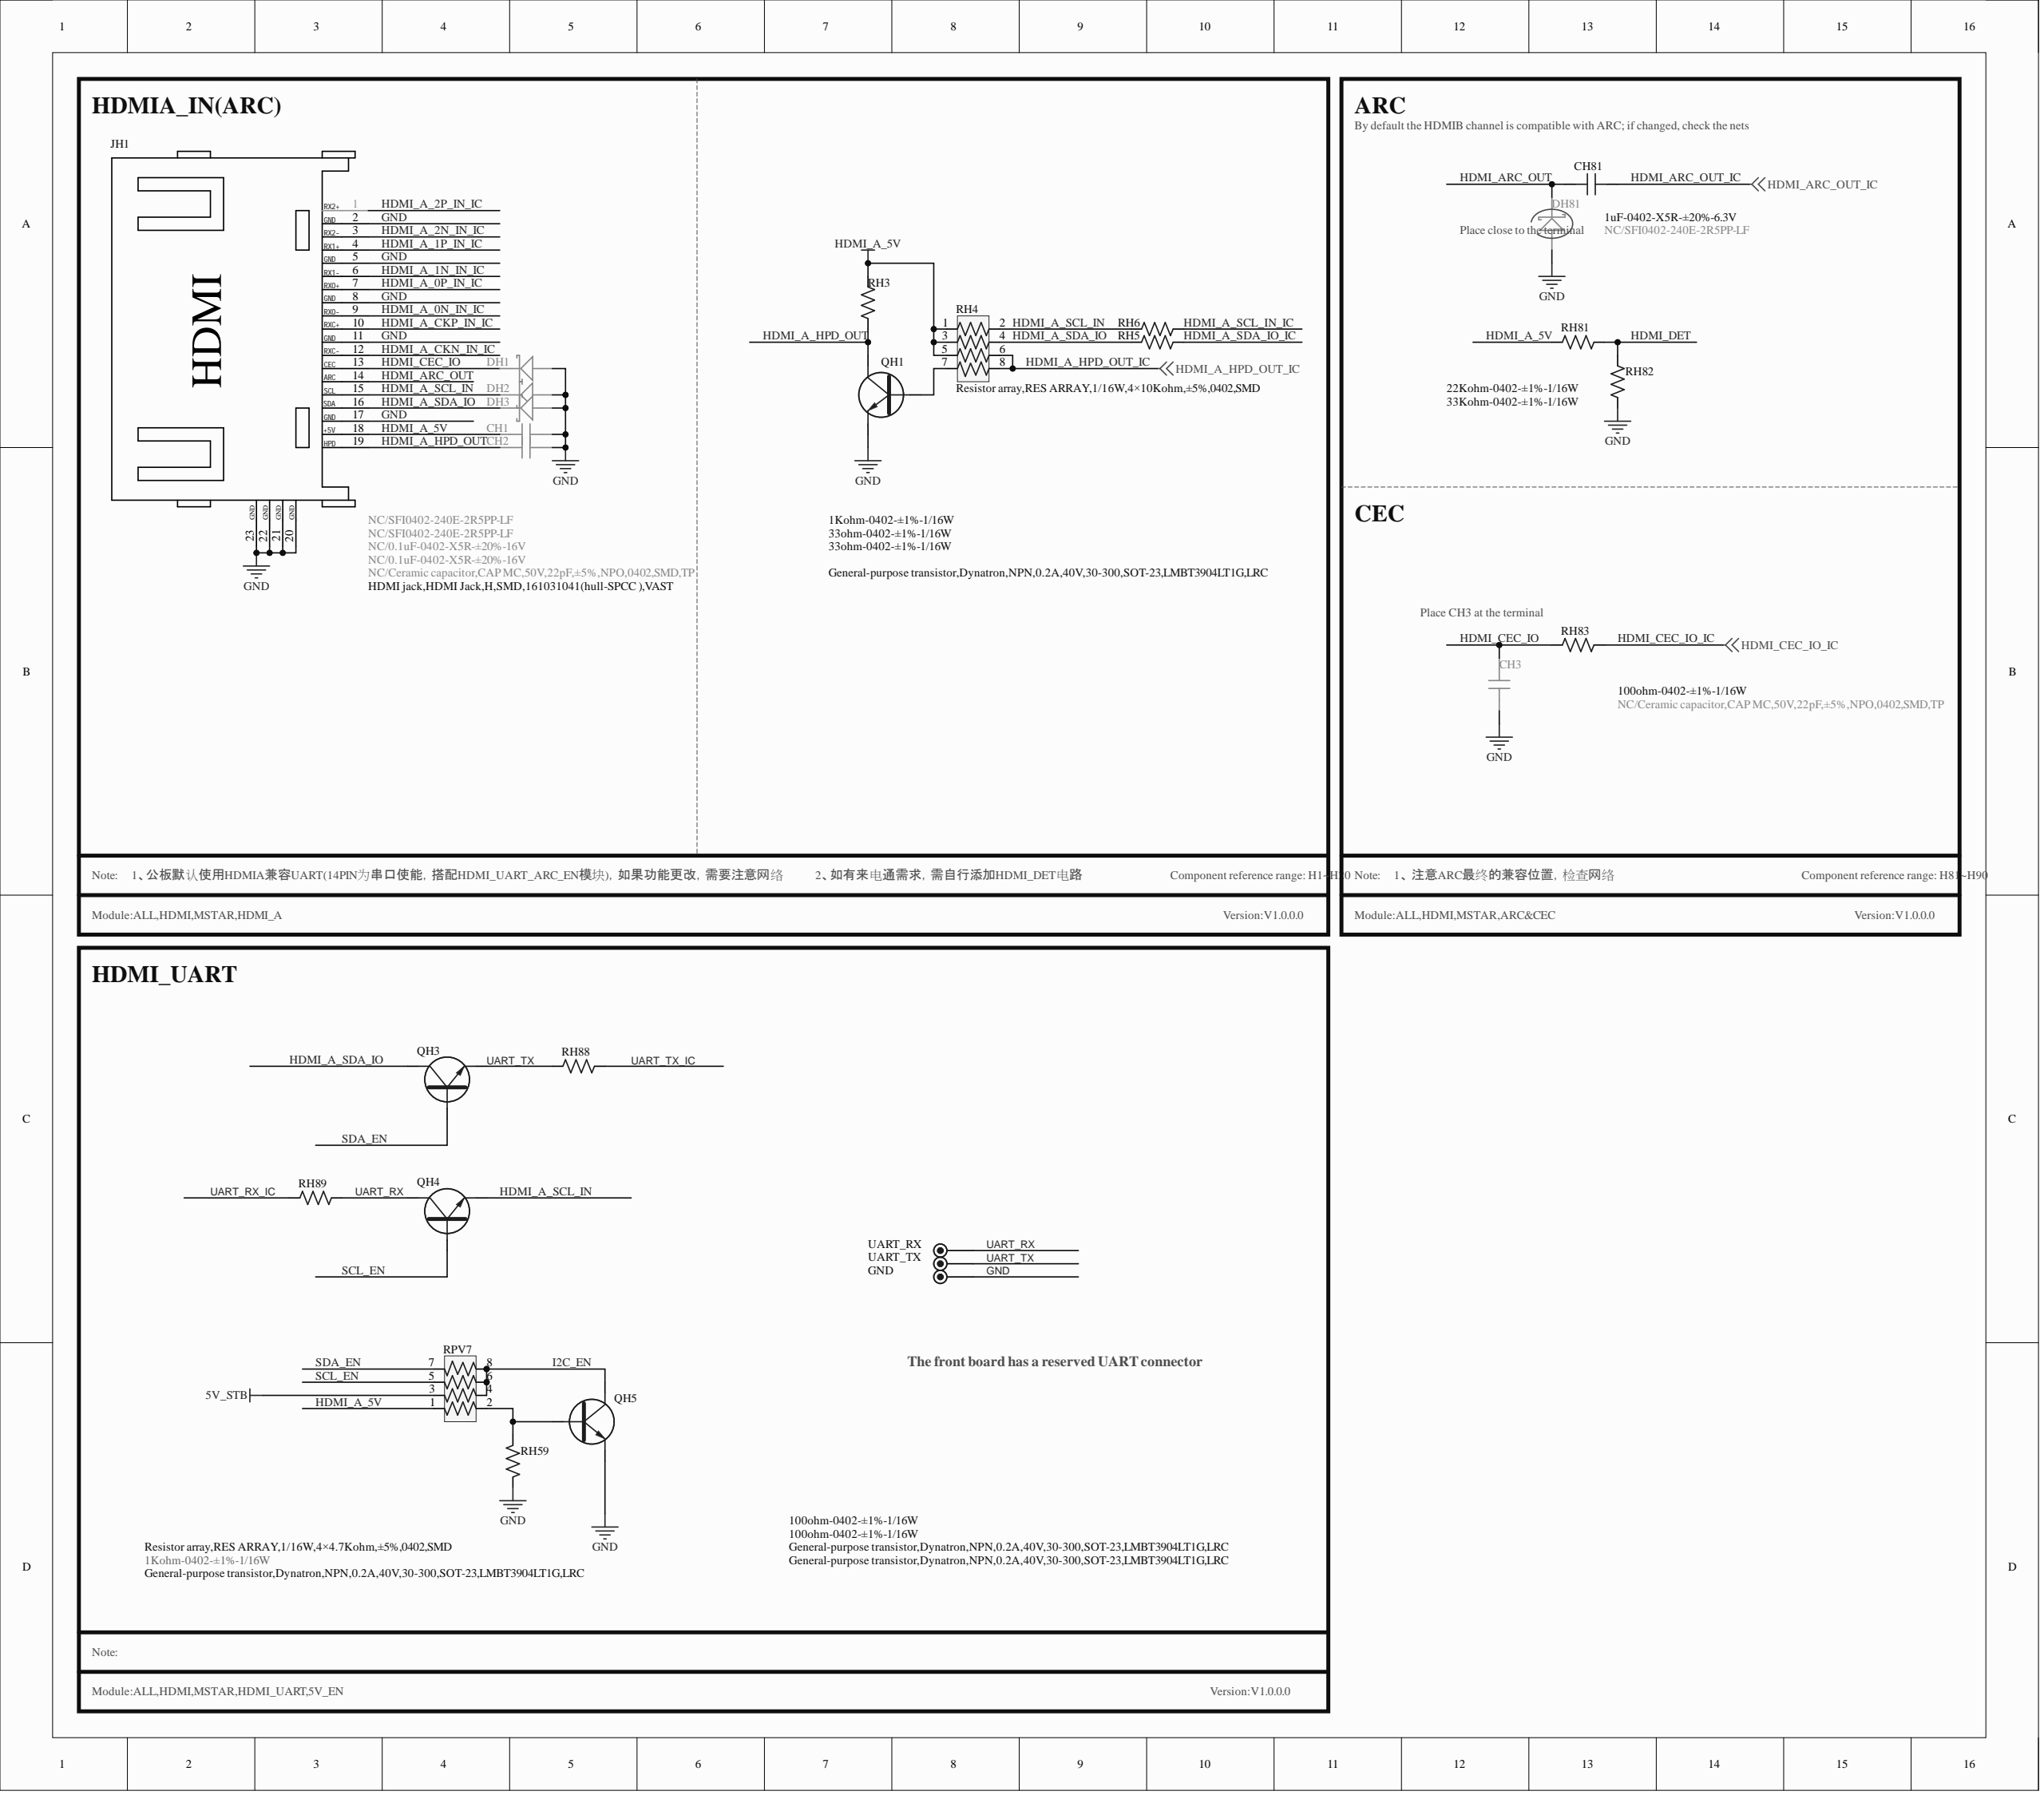Circuit board | Altium Designer | 527 parts | 243 nets | one sheet of the schematic
Parts on this sheet (reference | value | footprint):
CH1 | NC/0.1uF-0402-X5R-±20%-16V | C0402
CH2 | NC/0.1uF-0402-X5R-±20%-16V | C0402
CH3 | NC/Ceramic capacitor,CAP MC,50V,22pF,±5%,NPO,0402,SMD,TP | C0402
CH81 | 1uF-0402-X5R-±20%-6.3V | C0402
DH1 | NC/Ceramic capacitor,CAP MC,50V,22pF,±5%,NPO,0402,SMD,TP | DIODE-S0402
DH2 | NC/SFI0402-240E-2R5PP-LF | DIODE-S0402
DH3 | NC/SFI0402-240E-2R5PP-LF | DIODE-S0402
DH81 | NC/SFI0402-240E-2R5PP-LF | DIODE-S0402
JH1 | HDMI jack,HDMI Jack,H,SMD,161031041(hull-SPCC ),VAST | HDMI-HS-1
QH1 | General-purpose transistor,Dynatron,NPN,0.2A,40V,30-300,SOT-23,LMBT3904LT1G,LRC | SOT-23
QH3 | General-purpose transistor,Dynatron,NPN,0.2A,40V,30-300,SOT-23,LMBT3904LT1G,LRC | SOT-23
QH4 | General-purpose transistor,Dynatron,NPN,0.2A,40V,30-300,SOT-23,LMBT3904LT1G,LRC | SOT-23
QH5 | General-purpose transistor,Dynatron,NPN,0.2A,40V,30-300,SOT-23,LMBT3904LT1G,LRC | SOT-23
RH3 | 1Kohm-0402-±1%-1/16W | R0402
RH4 | Resistor array,RES ARRAY,1/16W,4×10Kohm,±5%,0402,SMD | RA0402
RH5 | 33ohm-0402-±1%-1/16W | R0402
RH6 | 33ohm-0402-±1%-1/16W | R0402
RH59 | 1Kohm-0402-±1%-1/16W | R0402
RH81 | 22Kohm-0402-±1%-1/16W | R0402
RH82 | 33Kohm-0402-±1%-1/16W | R0402
RH83 | 100ohm-0402-±1%-1/16W | R0402
RH88 | 100ohm-0402-±1%-1/16W | R0402
RH89 | 100ohm-0402-±1%-1/16W | R0402
RPV7 | Resistor array,RES ARRAY,1/16W,4×4.7Kohm,±5%,0402,SMD | RA0402
UART_RX | TP
UART_TX | TP
Nets of these parts (net: part-pin ...):
UART_TX_IC: RH88-1
UART_TX: QH3-E RH88-2 UART_TX-1
UART_RX_IC: RH89-2
UART_RX: QH4-C RH89-1 UART_RX-1
SDA_EN: QH3-B RPV7-7
SCL_EN: QH4-B RPV7-5
NetQH5_B: QH5-B RH59-2 RPV7-2
NetQH1_B: QH1-B RH4-7
I2C_EN: QH5-C RPV7-4 RPV7-6 RPV7-8
HDMI_DET: RH81-1 RH82-1
HDMI_CEC_IO_IC: RH83-1
HDMI_CEC_IO: CH3-2 DH1-K RH83-2 JH1-13
HDMI_ARC_OUT_IC: CH81-2
HDMI_ARC_OUT: CH81-1 DH81-K JH1-14
HDMI_A_SDA_IO_IC: RH5-2
HDMI_A_SDA_IO: DH3-K QH3-C RH4-4 RH5-1 JH1-16
HDMI_A_SCL_IN_IC: RH6-2
HDMI_A_SCL_IN: DH2-K QH4-E RH4-2 RH6-1 JH1-15
HDMI_A_HPD_OUT_IC: RH4-6 RH4-8
HDMI_A_HPD_OUT: CH2-1 QH1-C RH3-1 JH1-19
HDMI_A_CKP_IN_IC: JH1-10
HDMI_A_CKN_IN_IC: JH1-12
HDMI_A_5V: CH1-1 RH3-2 RH4-1 RH4-3 RH4-5 RH81-2 RPV7-1 JH1-18
HDMI_A_2P_IN_IC: JH1-1
HDMI_A_2N_IN_IC: JH1-3
HDMI_A_1P_IN_IC: JH1-4
HDMI_A_1N_IN_IC: JH1-6
HDMI_A_0P_IN_IC: JH1-7
HDMI_A_0N_IN_IC: JH1-9
GND: CH1-2 CH2-2 CH3-1 DH1-A DH2-A DH3-A DH81-A QH1-E QH5-E RH59-1 RH82-2 JH1-2 JH1-5 JH1-8 JH1-11 JH1-17 JH1-20 JH1-21 JH1-22 JH1-23
5V_STB: RPV7-3